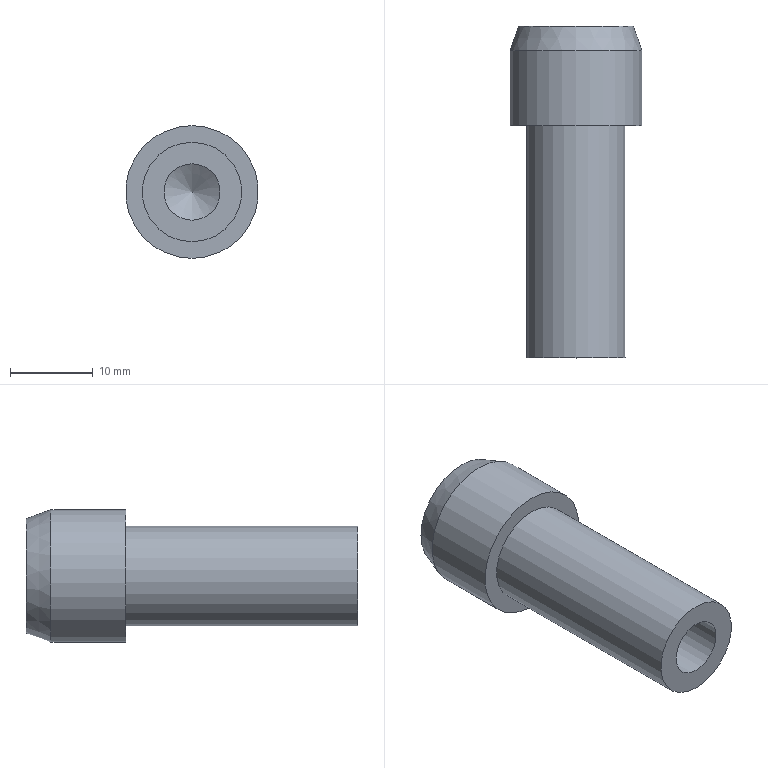Part | NX | features BREP 1 | 1 solid | 8 faces | box 16 x 40 x 16 mm | volume 4759 mm3 | plane 3 | cylinder 3 | cone 2 | commonest cylinder face diameters 6.8 x1 12 x1 16 x1
STEP:
#1=CARTESIAN_POINT('',(0.,0.,-3.4));
#2=VERTEX_POINT('',#1);
#3=CARTESIAN_POINT('',(0.,0.,0.));
#4=DIRECTION('',(0.,-1.,0.));
#5=DIRECTION('',(0.,0.,-1.));
#6=AXIS2_PLACEMENT_3D('',#3,#4,#5);
#7=CIRCLE('',#6,3.4);
#8=EDGE_CURVE('',#2,#2,#7,.T.);
#9=ORIENTED_EDGE('',*,*,#8,.F.);
#10=EDGE_LOOP('',(#9));
#11=FACE_BOUND('',#10,.T.);
#12=CARTESIAN_POINT('',(0.,0.,6.));
#13=VERTEX_POINT('',#12);
#14=CARTESIAN_POINT('',(0.,0.,0.));
#15=DIRECTION('',(0.,1.,0.));
#16=DIRECTION('',(0.,0.,1.));
#17=AXIS2_PLACEMENT_3D('',#14,#15,#16);
#18=CIRCLE('',#17,6.);
#19=EDGE_CURVE('',#13,#13,#18,.T.);
#20=ORIENTED_EDGE('',*,*,#19,.F.);
#21=EDGE_LOOP('',(#20));
#22=FACE_BOUND('',#21,.T.);
#23=CARTESIAN_POINT('',(0.,0.,0.));
#24=DIRECTION('',(0.,1.,0.));
#25=DIRECTION('',(0.,0.,-1.));
#26=AXIS2_PLACEMENT_3D('',#23,#24,#25);
#27=PLANE('',#26);
#28=ADVANCED_FACE('',(#11,#22),#27,.F.);
#29=CARTESIAN_POINT('',(0.,28.,6.));
#30=VERTEX_POINT('',#29);
#31=CARTESIAN_POINT('',(0.,28.,0.));
#32=DIRECTION('',(0.,1.,0.));
#33=DIRECTION('',(0.,0.,1.));
#34=AXIS2_PLACEMENT_3D('',#31,#32,#33);
#35=CIRCLE('',#34,6.);
#36=EDGE_CURVE('',#30,#30,#35,.T.);
#37=ORIENTED_EDGE('',*,*,#36,.F.);
#38=EDGE_LOOP('',(#37));
#39=FACE_BOUND('',#38,.T.);
#40=ORIENTED_EDGE('',*,*,#19,.T.);
#41=EDGE_LOOP('',(#40));
#42=FACE_BOUND('',#41,.T.);
#43=CARTESIAN_POINT('',(0.,0.,0.));
#44=DIRECTION('',(0.,1.,0.));
#45=DIRECTION('',(0.,0.,-1.));
#46=AXIS2_PLACEMENT_3D('',#43,#44,#45);
#47=CYLINDRICAL_SURFACE('',#46,6.);
#48=ADVANCED_FACE('',(#39,#42),#47,.T.);
#49=CARTESIAN_POINT('',(0.,28.,8.));
#50=VERTEX_POINT('',#49);
#51=CARTESIAN_POINT('',(0.,28.,0.));
#52=DIRECTION('',(0.,1.,0.));
#53=DIRECTION('',(0.,0.,1.));
#54=AXIS2_PLACEMENT_3D('',#51,#52,#53);
#55=CIRCLE('',#54,8.);
#56=EDGE_CURVE('',#50,#50,#55,.T.);
#57=ORIENTED_EDGE('',*,*,#56,.F.);
#58=EDGE_LOOP('',(#57));
#59=FACE_BOUND('',#58,.T.);
#60=ORIENTED_EDGE('',*,*,#36,.T.);
#61=EDGE_LOOP('',(#60));
#62=FACE_BOUND('',#61,.T.);
#63=CARTESIAN_POINT('',(6.,28.,0.));
#64=DIRECTION('',(0.,1.,0.));
#65=DIRECTION('',(0.,0.,-1.));
#66=AXIS2_PLACEMENT_3D('',#63,#64,#65);
#67=PLANE('',#66);
#68=ADVANCED_FACE('',(#59,#62),#67,.F.);
#69=CARTESIAN_POINT('',(0.,37.,8.));
#70=VERTEX_POINT('',#69);
#71=CARTESIAN_POINT('',(0.,37.,0.));
#72=DIRECTION('',(0.,1.,0.));
#73=DIRECTION('',(0.,0.,1.));
#74=AXIS2_PLACEMENT_3D('',#71,#72,#73);
#75=CIRCLE('',#74,8.);
#76=EDGE_CURVE('',#70,#70,#75,.T.);
#77=ORIENTED_EDGE('',*,*,#76,.F.);
#78=EDGE_LOOP('',(#77));
#79=FACE_BOUND('',#78,.T.);
#80=ORIENTED_EDGE('',*,*,#56,.T.);
#81=EDGE_LOOP('',(#80));
#82=FACE_BOUND('',#81,.T.);
#83=CARTESIAN_POINT('',(0.,0.,0.));
#84=DIRECTION('',(0.,1.,0.));
#85=DIRECTION('',(0.,0.,-1.));
#86=AXIS2_PLACEMENT_3D('',#83,#84,#85);
#87=CYLINDRICAL_SURFACE('',#86,8.);
#88=ADVANCED_FACE('',(#79,#82),#87,.T.);
#89=CARTESIAN_POINT('',(0.,40.,6.908));
#90=VERTEX_POINT('',#89);
#91=CARTESIAN_POINT('',(0.,40.,0.));
#92=DIRECTION('',(0.,1.,0.));
#93=DIRECTION('',(0.,0.,1.));
#94=AXIS2_PLACEMENT_3D('',#91,#92,#93);
#95=CIRCLE('',#94,6.908);
#96=EDGE_CURVE('',#90,#90,#95,.T.);
#97=ORIENTED_EDGE('',*,*,#96,.F.);
#98=EDGE_LOOP('',(#97));
#99=FACE_BOUND('',#98,.T.);
#100=ORIENTED_EDGE('',*,*,#76,.T.);
#101=EDGE_LOOP('',(#100));
#102=FACE_BOUND('',#101,.T.);
#103=CARTESIAN_POINT('',(0.,37.,0.));
#104=DIRECTION('',(0.,-1.,0.));
#105=DIRECTION('',(0.,0.,1.));
#106=AXIS2_PLACEMENT_3D('',#103,#104,#105);
#107=CONICAL_SURFACE('',#106,8.,0.3491);
#108=ADVANCED_FACE('',(#99,#102),#107,.T.);
#109=ORIENTED_EDGE('',*,*,#96,.T.);
#110=EDGE_LOOP('',(#109));
#111=FACE_BOUND('',#110,.T.);
#112=CARTESIAN_POINT('',(6.908,40.,0.));
#113=DIRECTION('',(0.,-1.,0.));
#114=DIRECTION('',(0.,0.,1.));
#115=AXIS2_PLACEMENT_3D('',#112,#113,#114);
#116=PLANE('',#115);
#117=ADVANCED_FACE('',(#111),#116,.F.);
#118=CARTESIAN_POINT('',(0.,21.793,0.));
#119=VERTEX_POINT('',#118);
#120=VERTEX_LOOP('',#119);
#121=FACE_BOUND('',#120,.T.);
#122=CARTESIAN_POINT('',(0.,19.75,-3.4));
#123=VERTEX_POINT('',#122);
#124=CARTESIAN_POINT('',(0.,19.75,0.));
#125=DIRECTION('',(0.,-1.,0.));
#126=DIRECTION('',(0.,0.,-1.));
#127=AXIS2_PLACEMENT_3D('',#124,#125,#126);
#128=CIRCLE('',#127,3.4);
#129=EDGE_CURVE('',#123,#123,#128,.T.);
#130=ORIENTED_EDGE('',*,*,#129,.T.);
#131=EDGE_LOOP('',(#130));
#132=FACE_BOUND('',#131,.T.);
#133=CARTESIAN_POINT('',(0.,19.75,0.));
#134=DIRECTION('',(0.,-1.,0.));
#135=DIRECTION('',(0.,0.,1.));
#136=AXIS2_PLACEMENT_3D('',#133,#134,#135);
#137=CONICAL_SURFACE('',#136,3.4,1.03);
#138=ADVANCED_FACE('',(#121,#132),#137,.F.);
#139=ORIENTED_EDGE('',*,*,#129,.F.);
#140=EDGE_LOOP('',(#139));
#141=FACE_BOUND('',#140,.T.);
#142=ORIENTED_EDGE('',*,*,#8,.T.);
#143=EDGE_LOOP('',(#142));
#144=FACE_BOUND('',#143,.T.);
#145=CARTESIAN_POINT('',(0.,0.,0.));
#146=DIRECTION('',(0.,-1.,0.));
#147=DIRECTION('',(0.,0.,1.));
#148=AXIS2_PLACEMENT_3D('',#145,#146,#147);
#149=CYLINDRICAL_SURFACE('',#148,3.4);
#150=ADVANCED_FACE('',(#141,#144),#149,.F.);
#151=CLOSED_SHELL('',(#28,#48,#68,#88,#108,#117,#138,#150));
#152=MANIFOLD_SOLID_BREP('',#151);
#153=(LENGTH_UNIT()NAMED_UNIT(*)SI_UNIT(.MILLI.,.METRE.));
#154=UNCERTAINTY_MEASURE_WITH_UNIT(LENGTH_MEASURE(0.00001),#153,'','');
#155=(NAMED_UNIT(*)PLANE_ANGLE_UNIT()SI_UNIT($,.RADIAN.));
#156=(NAMED_UNIT(*)SI_UNIT($,.STERADIAN.)SOLID_ANGLE_UNIT());
#157=(GEOMETRIC_REPRESENTATION_CONTEXT(3)GLOBAL_UNCERTAINTY_ASSIGNED_CONTEXT((#154))GLOBAL_UNIT_ASSIGNED_CONTEXT((#153,#155,#156))REPRESENTATION_CONTEXT('',''));
#158=ADVANCED_BREP_SHAPE_REPRESENTATION('',(#152),#157);